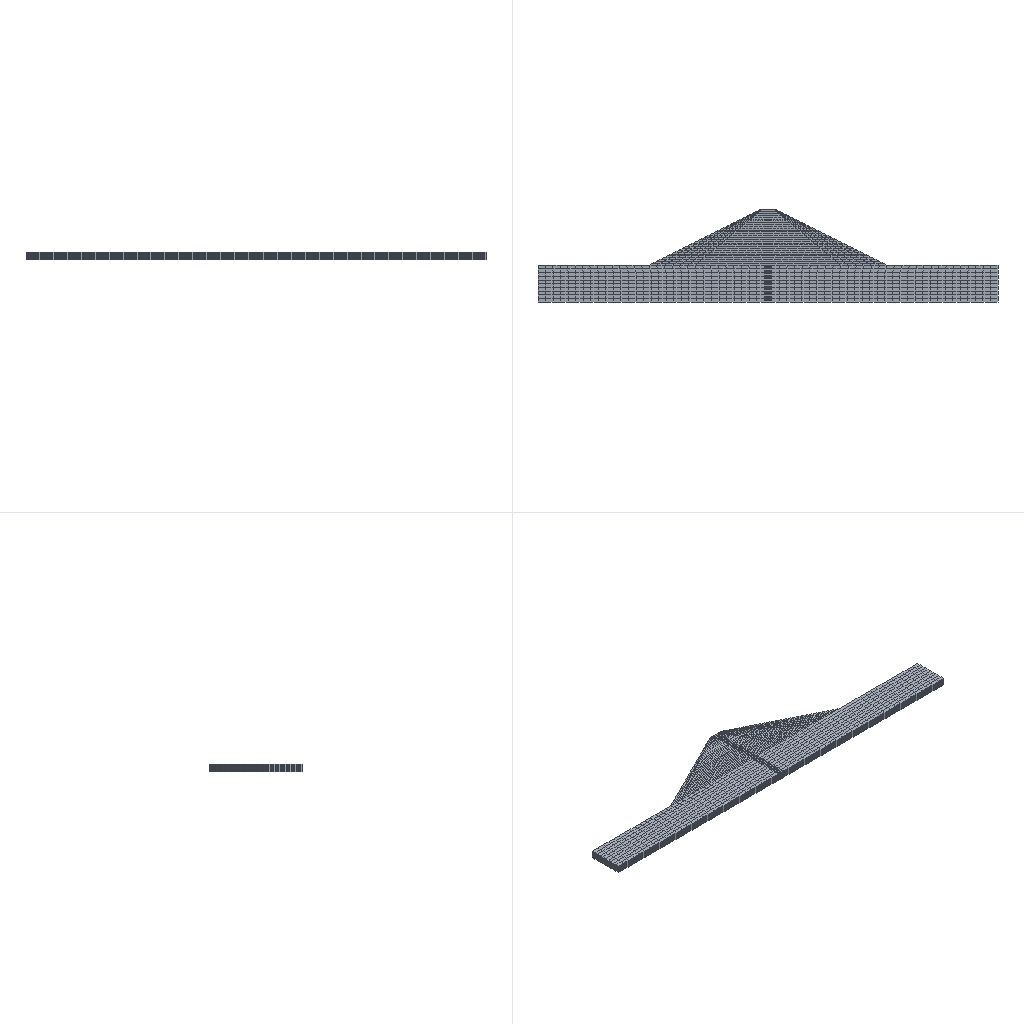Simulation study | abaqus
Set-up summary:
category,name,step,type,value,unit,region
solver,abaqus
solver,version,,,Abaqus/Standard 2020
units,not stated in the deck,,not stated
analysis,deck,,soils,soils
load_step,shenliu,shenliu,soils
load_step,requested,,,1
mesh,nodes,,,22968
mesh,elements,,,19240
element_type,C3D8P,,solid,19240
load,load commands in deck,,count,299
bc,support commands in deck,,count,313
material,BAJI,,in results
material,BATI,,in results
material,QIANG,,in results
check,setup vs results,,match,"per instance, exact: element labels, types and connectivity; labels of the nodes the elements use; coordinates of those nodes at SINGLE_PRECISION in 2 of 2 instance(s)"
Abaqus input file, long lists of numbers shortened:
*Heading
** Job name: Job-9 Model name: 3cm14mML300-OH-shenliu
** Generated by: Abaqus/CAE 2020
*Preprint, echo=NO, model=NO, history=NO, contact=NO
**
** PARTS
**
*Part, name=ba
*End Part
**
*Part, name=qiang
*End Part
**
**
** ASSEMBLY
**
*Assembly, name=Assembly
**
*Instance, name=ba-1, part=ba
*Node
      1,         67.5,         23.5,   1.2
      2,         67.5,         23.5,  0.9
** (22570 more lines like these left out)
*Element, type=C3D8P
 1,   208,  2707, 12325,  2651,     1,   169,  2647,   174
 2,  2707,   236,  2679, 12325,   169,     2,   170,  2647
** (19078 more lines like these left out)
*Nset, nset=Set-1
     1,     2,     3,     4,     5,     6,     7,     8,     9,    10,    11,    12,    13,    14,    15,    16
    17,    18,    19,    20,    21,    22,    23,    24,    25,    26,    27,    28,    29,    30,    31,    32
** (894 more lines like these left out)
*Elset, elset=Set-1
     1,     2,     3,     4,     5,     6,     7,     8,     9,    10,    11,    12,    13,    14,    15,    16
    17,    18,    19,    20,    21,    22,    23,    24,    25,    26,    27,    28,    29,    30,    31,    32
** (748 more lines like these left out)
*Nset, nset=Set-2
    18,    19,    21,    22,    24,    25,    26,    27,    41,    42,    44,    45,    56,    57,    59,    60
    75,    76,    77,    78,    79,    80,    81,    82,    83,    84,    85,    86,    87,    88,    89,    90
** (543 more lines like these left out)
*Elset, elset=Set-2
  4849,  4850,  4851,  4852,  4853,  4854,  4855,  4856,  4857,  4858,  4859,  4860,  4861,  4862,  4863,  4864
  4865,  4866,  4867,  4868,  4869,  4870,  4871,  4872,  4873,  4874,  4875,  4876,  4877,  4878,  4879,  4880
** (441 more lines like these left out)
** Section: bati
*Solid Section, elset=Set-1, material=bati
,
** Section: baji
*Solid Section, elset=Set-2, material=baji
,
*End Instance
**
*Instance, name=qiang-1, part=qiang
      62.235,           8.,           0.
*Node
      1, 0.03,         15.5,           0.
      2, 0.03,         15.5,  0.9
** (394 more lines like these left out)
*Element, type=C3D8P
 1,   8,  87, 307, 115,   1,  33, 281,  86
 2,  87,   5, 113, 307,  33,   2,  34, 281
** (158 more lines like these left out)
*Nset, nset=Set-1, generate
   1,  396,    1
*Elset, elset=Set-1, generate
   1,  160,    1
** Section: qiang
*Solid Section, elset=Set-1, material=qiang
,
*End Instance
**
*Nset, nset=Set-1, instance=ba-1
    18,    19,    21,    22,    24,    25,    26,    27,    41,    42,    44,    45,    56,    57,    59,    60
    75,    76,    77,    78,    79,    80,    81,    82,    83,    84,    85,    86,    87,    88,    89,    90
** (543 more lines like these left out)
*Elset, elset=Set-1, instance=ba-1
  4849,  4850,  4851,  4852,  4853,  4854,  4855,  4856,  4857,  4858,  4859,  4860,  4861,  4862,  4863,  4864
  4865,  4866,  4867,  4868,  4869,  4870,  4871,  4872,  4873,  4874,  4875,  4876,  4877,  4878,  4879,  4880
** (441 more lines like these left out)
*Nset, nset=Set-2, instance=ba-1
   115,   116,   117,   118,   121,   122,   125,   126,   135,   136,   137,   138,   145,   146,   149,   150
   156,   157,   158,   159,   162,   163,   164,   165,  1335,  1336,  1337,  1338,  1444,  1445,  1446,  1447
** (14 more lines like these left out)
*Elset, elset=Set-2, instance=ba-1
  5525,  5526,  5527,  5528,  5761,  5762,  5763,  5764,  5765,  5766,  5767,  5768,  6001,  6002,  6003,  6004
  6005,  6006,  6007,  6008,  6553,  6554,  6555,  6556,  6557,  6558,  6559,  6560,  6561,  6562,  6563,  6564
** (11 more lines like these left out)
*Nset, nset=Set-3, instance=ba-1
    81,    82,    83,    84,    85,    88,    91,    92,    93,    94,    97,    98,   127,   128,   129,   130
   133,   134,   136,   137,   140,   141,   142,   144,   145,   147,   148,   150,   162,   163,   164,   165
** (48 more lines like these left out)
*Elset, elset=Set-3, instance=ba-1
  4877,  4878,  4879,  4880,  4881,  4889,  4897,  4905,  4927,  4928,  4929,  4930,  4931,  4932,  4933,  4934
  4935,  4936,  4937,  4938,  4939,  4940,  4941,  4942,  4943,  4944,  5057,  5058,  5059,  5060,  5061,  5062
** (43 more lines like these left out)
*Nset, nset=Set-4, instance=ba-1
    17,    19,    20,    22,    23,    25,    27,    28,    29,    30,    31,    32,    35,    36,    37,    38
    39,    40,    41,    42,    51,    52,    53,    54,    58,    60,    63,    64,    65,    66,    67,    68
** (255 more lines like these left out)
*Nset, nset=Set-4, instance=qiang-1
   1,   4,   7,   8,   9,  12,  15,  16,  22,  23,  27,  28,  29,  30,  31,  32
  61,  62,  63,  64,  65,  66,  67,  68,  69,  70,  71,  72,  73,  74,  75,  76
** (7 more lines like these left out)
*Elset, elset=Set-4, instance=ba-1
   181,   185,   189,   193,   197,   201,   205,   209,   213,   217,   221,   225,   229,   233,   237,   241
   245,   249,   253,   257,   261,   265,   269,   273,   277,   281,   285,   289,   293,   297,   301,   305
** (237 more lines like these left out)
*Elset, elset=Set-4, instance=qiang-1
   1,   3,   5,   7,   9,  11,  13,  15,  17,  19,  21,  23,  25,  27,  29,  31
  33,  35,  37,  39,  41,  43,  45,  47,  49,  51,  53,  55,  57,  59,  93,  94
** (2 more lines like these left out)
*Nset, nset=Set-6, instance=ba-1
     1,     2,     3,     4,     6,     7,    13,    14,    15,    16,    18,    19,    20,    21,    22,    24
    25,    26,    27,    28,    31,    32,    34,    36,    37,    41,    42,    44,    45,    49,    53,    56
** (599 more lines like these left out)
*Nset, nset=Set-6, instance=qiang-1
   1,   4,   7,   8,  11,  12,  14,  15,  17,  18,  21,  22,  23,  24,  25,  26
  29,  30,  31,  32,  61,  62,  63,  64,  65,  66,  67,  68,  69,  70,  71,  72
** (4 more lines like these left out)
*Elset, elset=Set-6, instance=ba-1
     1,     2,     3,     4,     5,     6,    11,    12,    17,    18,    23,    24,    29,    30,    35,    36
    41,    42,    47,    48,    53,    54,    59,    60,    65,    66,    71,    72,    77,    78,    83,    84
** (491 more lines like these left out)
*Elset, elset=Set-6, instance=qiang-1
   1,   3,   5,   7,   9,  11,  13,  15,  17,  19,  21,  23,  25,  27,  29,  31
  33,  35,  37,  39,  41,  43,  45,  47,  49,  51,  53,  59,  60,  63,  91,  93
** (1 more lines like these left out)
*Nset, nset=Set-7, instance=ba-1, generate
     1,  22572,      1
*Nset, nset=Set-7, instance=qiang-1, generate
   1,  396,    1
*Elset, elset=Set-7, instance=ba-1, generate
     1,  19080,      1
*Elset, elset=Set-7, instance=qiang-1, generate
   1,  160,    1
*Nset, nset=Set-8, instance=ba-1
    18,    19,    21,    22,    24,    25,    26,    27,    41,    42,    44,    45,    56,    57,    59,    60
    75,    76,    77,    78,    79,    80,    81,    82,    83,    84,    85,    86,    87,    88,    89,    90
** (543 more lines like these left out)
*Elset, elset=Set-8, instance=ba-1
  4849,  4850,  4851,  4852,  4853,  4854,  4855,  4856,  4857,  4858,  4859,  4860,  4861,  4862,  4863,  4864
  4865,  4866,  4867,  4868,  4869,  4870,  4871,  4872,  4873,  4874,  4875,  4876,  4877,  4878,  4879,  4880
** (441 more lines like these left out)
*Nset, nset=Set-9, instance=ba-1
    18,    19,    21,    22,    24,    25,    26,    27,    41,    42,    44,    45,    56,    57,    59,    60
    75,    76,    77,    78,    79,    80,    81,    82,    83,    84,    85,    86,    87,    88,    89,    90
** (543 more lines like these left out)
*Elset, elset=Set-9, instance=ba-1
  4849,  4850,  4851,  4852,  4853,  4854,  4855,  4856,  4857,  4858,  4859,  4860,  4861,  4862,  4863,  4864
  4865,  4866,  4867,  4868,  4869,  4870,  4871,  4872,  4873,  4874,  4875,  4876,  4877,  4878,  4879,  4880
** (441 more lines like these left out)
*Nset, nset=Set-10, instance=ba-1
    18,    19,    21,    22,    24,    25,    26,    27,    41,    42,    44,    45,    56,    57,    59,    60
    75,    76,    77,    78,    79,    80,    81,    82,    83,    84,    85,    86,    87,    88,    89,    90
** (543 more lines like these left out)
*Elset, elset=Set-10, instance=ba-1
  4849,  4850,  4851,  4852,  4853,  4854,  4855,  4856,  4857,  4858,  4859,  4860,  4861,  4862,  4863,  4864
  4865,  4866,  4867,  4868,  4869,  4870,  4871,  4872,  4873,  4874,  4875,  4876,  4877,  4878,  4879,  4880
** (441 more lines like these left out)
*Nset, nset=Set-12, instance=ba-1
    13,    14,    20,    21,    22,    32,   119,   123,   243,   363,   364,   365,   366,   367,   368,   369
   370,   371,   372,   373,   374,   375,   376,   377,   378,   379,   380,   381,   382,   383,   384,   385
** (18 more lines like these left out)
*Elset, elset=Set-12, instance=ba-1
  1693,  1694,  1695,  1696,  1697,  1698,  1699,  1700,  1701,  1702,  1703,  1704,  1705,  1706,  1707,  1708
  1709,  1710,  1711,  1712,  1713,  1714,  1715,  1716,  1717,  1718,  1719,  1720,  1721,  1722,  1723,  1724
** (15 more lines like these left out)
*Nset, nset=Set-15, instance=ba-1
    18,    19,    21,    22,    24,    25,    26,    27,    41,    42,    44,    45,    56,    57,    59,    60
    75,    76,    77,    78,    79,    80,    81,    82,    83,    84,    85,    86,    87,    88,    89,    90
** (543 more lines like these left out)
*Elset, elset=Set-15, instance=ba-1
  4849,  4850,  4851,  4852,  4853,  4854,  4855,  4856,  4857,  4858,  4859,  4860,  4861,  4862,  4863,  4864
  4865,  4866,  4867,  4868,  4869,  4870,  4871,  4872,  4873,  4874,  4875,  4876,  4877,  4878,  4879,  4880
** (441 more lines like these left out)
*Nset, nset=Set-21, instance=ba-1
    18,    19,    21,    22,    24,    25,    26,    27,    41,    42,    44,    45,    56,    57,    59,    60
    75,    76,    77,    78,    79,    80,    81,    82,    83,    84,    85,    86,    87,    88,    89,    90
** (543 more lines like these left out)
*Elset, elset=Set-21, instance=ba-1
  4849,  4850,  4851,  4852,  4853,  4854,  4855,  4856,  4857,  4858,  4859,  4860,  4861,  4862,  4863,  4864
  4865,  4866,  4867,  4868,  4869,  4870,  4871,  4872,  4873,  4874,  4875,  4876,  4877,  4878,  4879,  4880
** (441 more lines like these left out)
*Nset, nset=Set-22, instance=ba-1
    18,    19,    21,    22,    24,    25,    26,    27,    41,    42,    44,    45,    56,    57,    59,    60
    75,    76,    77,    78,    79,    80,    81,    82,    83,    84,    85,    86,    87,    88,    89,    90
** (543 more lines like these left out)
*Elset, elset=Set-22, instance=ba-1
  4849,  4850,  4851,  4852,  4853,  4854,  4855,  4856,  4857,  4858,  4859,  4860,  4861,  4862,  4863,  4864
  4865,  4866,  4867,  4868,  4869,  4870,  4871,  4872,  4873,  4874,  4875,  4876,  4877,  4878,  4879,  4880
** (441 more lines like these left out)
*Nset, nset=Set-23, instance=ba-1, generate
     1,  22572,      1
*Nset, nset=Set-23, instance=qiang-1, generate
   1,  396,    1
*Elset, elset=Set-23, instance=ba-1, generate
     1,  19080,      1
*Elset, elset=Set-23, instance=qiang-1, generate
   1,  160,    1
*Elset, elset=_ba-xia_S2, internal, instance=ba-1
 4849, 4850, 4851, 4852, 4913, 4914
*Elset, elset=_ba-xia_S4, internal, instance=ba-1, generate
 4888,  4912,     8
*Surface, type=ELEMENT, name=ba-xia
_ba-xia_S2, S2
_ba-xia_S4, S4
*Elset, elset=_ba-you_S5, internal, instance=ba-1
  5261,  5262,  5263,  5264,  5277,  5278,  5279,  5280,  5325,  5326,  5327,  5328,  5341,  5342,  5343,  5344
  5383,  5384,  5391,  5392, 10983, 10984, 10985, 10986, 10999, 11000, 11001, 11002, 11015, 11016, 11017, 11018
** (13 more lines like these left out)
*Elset, elset=_ba-you_S4, internal, instance=ba-1, generate
 10510,  10722,      4
*Elset, elset=_ba-you_S2, internal, instance=ba-1, generate
 4549,  4554,     1
*Elset, elset=_ba-you_S6, internal, instance=ba-1, generate
 4435,  4527,     4
*Surface, type=ELEMENT, name=ba-you
_ba-you_S5, S5
_ba-you_S4, S4
_ba-you_S2, S2
_ba-you_S6, S6
*Elset, elset=_ba-zuo_S4, internal, instance=ba-1, generate
 3616,  4092,     4
*Elset, elset=_ba-zuo_S6, internal, instance=ba-1, generate
 4099,  4311,     4
*Elset, elset=_ba-zuo_S5, internal, instance=ba-1
 12101, 12102, 12109, 12110, 12117, 12118, 14105, 14106, 14107, 14108, 14121, 14122, 14123, 14124, 14137, 14138
 14139, 14140, 14153, 14154, 14155, 14156, 14169, 14170, 14171, 14172, 14185, 14186, 14187, 14188, 14201, 14202
** (6 more lines like these left out)
*Elset, elset=_ba-zuo_S1, internal, instance=ba-1
 5305, 5306, 5307, 5308, 5309, 5310, 5311, 5312, 5369, 5370, 5371, 5372, 5373, 5374, 5375, 5376
 5405, 5406, 5407, 5408
*Surface, type=ELEMENT, name=ba-zuo
_ba-zuo_S4, S4
_ba-zuo_S6, S6
_ba-zuo_S5, S5
_ba-zuo_S1, S1
*Elset, elset=_baxia_S1, internal, instance=ba-1
  3313,  3314,  3315,  3316,  3317,  3318,  3319,  3320,  3321,  3322,  3323,  3324,  3325,  3326,  3327,  3328
  3329,  3330,  3331,  3332,  3333,  3334,  3335,  3336,  3337,  3338,  3339,  3340,  3341,  3342,  3343,  3344
** (6 more lines like these left out)
*Elset, elset=_baxia_S2, internal, instance=ba-1, generate
 1,  6,  1
*Elset, elset=_baxia_S6, internal, instance=ba-1
  4555,  4570,  4585,  4600,  4615,  4630,  4645,  4660,  4675,  4690,  4705,  4720, 18271, 18286, 18301, 18316
 18331, 18346, 18361, 18376, 18391, 18406, 18421, 18436, 18451, 18466, 18481, 18496, 18511, 18526, 18541, 18556
** (3 more lines like these left out)
*Elset, elset=_baxia_S5, internal, instance=ba-1
  8691,  8692,  8693,  8694,  8751,  8752,  8753,  8754,  8811,  8812,  8813,  8814,  8871,  8872,  8873,  8874
  8931,  8932,  8933,  8934,  8991,  8992,  8993,  8994,  9051,  9052,  9053,  9054,  9111,  9112,  9113,  9114
** (5 more lines like these left out)
*Surface, type=ELEMENT, name=baxia
_baxia_S1, S1
_baxia_S2, S2
_baxia_S6, S6
_baxia_S5, S5
*Elset, elset=_fdown_S1, internal, instance=ba-1
  3313,  3314,  3315,  3316,  3317,  3318,  3319,  3320,  3321,  3322,  3323,  3324,  3325,  3326,  3327,  3328
  3329,  3330,  3331,  3332,  3333,  3334,  3335,  3336,  3337,  3338,  3339,  3340,  3341,  3342,  3343,  3344
** (6 more lines like these left out)
*Elset, elset=_fdown_S2, internal, instance=ba-1, generate
 1,  6,  1
*Elset, elset=_fdown_S6, internal, instance=ba-1
  4555,  4570,  4585,  4600,  4615,  4630,  4645,  4660,  4675,  4690,  4705,  4720, 18271, 18286, 18301, 18316
 18331, 18346, 18361, 18376, 18391, 18406, 18421, 18436, 18451, 18466, 18481, 18496, 18511, 18526, 18541, 18556
** (3 more lines like these left out)
*Elset, elset=_fdown_S5, internal, instance=ba-1
  8691,  8692,  8693,  8694,  8751,  8752,  8753,  8754,  8811,  8812,  8813,  8814,  8871,  8872,  8873,  8874
  8931,  8932,  8933,  8934,  8991,  8992,  8993,  8994,  9051,  9052,  9053,  9054,  9111,  9112,  9113,  9114
** (5 more lines like these left out)
*Surface, type=ELEMENT, name=fdown
_fdown_S1, S1
_fdown_S2, S2
_fdown_S6, S6
_fdown_S5, S5
*Elset, elset=_m_Surf-14_S4, internal, instance=ba-1, generate
 3616,  4092,     4
*Elset, elset=_m_Surf-14_S6, internal, instance=ba-1, generate
 4099,  4311,     4
*Elset, elset=_m_Surf-14_S5, internal, instance=ba-1
 12101, 12102, 12109, 12110, 12117, 12118, 14105, 14106, 14107, 14108, 14121, 14122, 14123, 14124, 14137, 14138
 14139, 14140, 14153, 14154, 14155, 14156, 14169, 14170, 14171, 14172, 14185, 14186, 14187, 14188, 14201, 14202
** (6 more lines like these left out)
*Elset, elset=_m_Surf-14_S1, internal, instance=ba-1
 5305, 5306, 5307, 5308, 5309, 5310, 5311, 5312, 5369, 5370, 5371, 5372, 5373, 5374, 5375, 5376
 5405, 5406, 5407, 5408
*Surface, type=ELEMENT, name=m_Surf-14
_m_Surf-14_S4, S4
_m_Surf-14_S6, S6
_m_Surf-14_S5, S5
_m_Surf-14_S1, S1
*Elset, elset=_m_Surf-16_S5, internal, instance=ba-1
  5261,  5262,  5263,  5264,  5277,  5278,  5279,  5280,  5325,  5326,  5327,  5328,  5341,  5342,  5343,  5344
  5383,  5384,  5391,  5392, 10983, 10984, 10985, 10986, 10999, 11000, 11001, 11002, 11015, 11016, 11017, 11018
** (13 more lines like these left out)
*Elset, elset=_m_Surf-16_S4, internal, instance=ba-1, generate
 10510,  10722,      4
*Elset, elset=_m_Surf-16_S2, internal, instance=ba-1, generate
 4549,  4554,     1
*Elset, elset=_m_Surf-16_S6, internal, instance=ba-1, generate
 4435,  4527,     4
*Surface, type=ELEMENT, name=m_Surf-16
_m_Surf-16_S5, S5
_m_Surf-16_S4, S4
_m_Surf-16_S2, S2
_m_Surf-16_S6, S6
*Elset, elset=_m_Surf-18_S2, internal, instance=ba-1
 4849, 4850, 4851, 4852, 4913, 4914
*Elset, elset=_m_Surf-18_S4, internal, instance=ba-1, generate
 4888,  4912,     8
*Surface, type=ELEMENT, name=m_Surf-18
_m_Surf-18_S2, S2
_m_Surf-18_S4, S4
*Elset, elset=_qiang-xia_S6, internal, instance=qiang-1
 91, 93
*Elset, elset=_qiang-xia_S4, internal, instance=qiang-1
  96, 158, 160
*Surface, type=ELEMENT, name=qiang-xia
_qiang-xia_S6, S6
_qiang-xia_S4, S4
*Elset, elset=_qiang-you_S2, internal, instance=qiang-1
   1,   2,   3,   4,   5,   6,   7,   8,   9,  10,  11,  12,  13,  14,  15,  16
  17,  18,  19,  20,  21,  22,  23,  24,  25,  26,  27,  28,  29,  30,  31,  32
** (8 more lines like these left out)
*Elset, elset=_qiang-you_S1, internal, instance=qiang-1
  91,  92,  93,  94,  95,  96, 157, 158, 159, 160
*Surface, type=ELEMENT, name=qiang-you
_qiang-you_S2, S2
_qiang-you_S1, S1
*Elset, elset=_qiang-zuo_S1, internal, instance=qiang-1
   1,   2,   3,   4,   5,   6,   7,   8,   9,  10,  11,  12,  13,  14,  15,  16
  17,  18,  19,  20,  21,  22,  23,  24,  25,  26,  27,  28,  29,  30,  31,  32
** (8 more lines like these left out)
*Elset, elset=_qiang-zuo_S2, internal, instance=qiang-1
  91,  92,  93,  94,  95,  96, 157, 158, 159, 160
*Surface, type=ELEMENT, name=qiang-zuo
_qiang-zuo_S1, S1
_qiang-zuo_S2, S2
*Elset, elset=_qiangdi_S5, internal, instance=qiang-1
  59,  60,  63, 155, 156
*Surface, type=ELEMENT, name=qiangdi
_qiangdi_S5, S5
*Elset, elset=_s_Surf-14_S1, internal, instance=qiang-1
   1,   2,   3,   4,   5,   6,   7,   8,   9,  10,  11,  12,  13,  14,  15,  16
  17,  18,  19,  20,  21,  22,  23,  24,  25,  26,  27,  28,  29,  30,  31,  32
** (8 more lines like these left out)
*Elset, elset=_s_Surf-14_S2, internal, instance=qiang-1
  91,  92,  93,  94,  95,  96, 157, 158, 159, 160
*Surface, type=ELEMENT, name=s_Surf-14
_s_Surf-14_S1, S1
_s_Surf-14_S2, S2
*Elset, elset=_s_Surf-16_S2, internal, instance=qiang-1
   1,   2,   3,   4,   5,   6,   7,   8,   9,  10,  11,  12,  13,  14,  15,  16
  17,  18,  19,  20,  21,  22,  23,  24,  25,  26,  27,  28,  29,  30,  31,  32
** (8 more lines like these left out)
*Elset, elset=_s_Surf-16_S1, internal, instance=qiang-1
  91,  92,  93,  94,  95,  96, 157, 158, 159, 160
*Surface, type=ELEMENT, name=s_Surf-16
_s_Surf-16_S2, S2
_s_Surf-16_S1, S1
*Elset, elset=_s_Surf-18_S6, internal, instance=qiang-1
 91, 93
*Elset, elset=_s_Surf-18_S4, internal, instance=qiang-1
  96, 158, 160
*Surface, type=ELEMENT, name=s_Surf-18
_s_Surf-18_S6, S6
_s_Surf-18_S4, S4
*Nset, nset=Set-12_PP_, internal, instance=ba-1
    13,    14,    20,    21,    22,    32,   119,   123,   243,   363,   364,   365,   366,   367,   368,   369
   370,   371,   372,   373,   374,   375,   376,   377,   378,   379,   380,   381,   382,   383,   384,   385
** (18 more lines like these left out)
*End Assembly
**
** MATERIALS
**
*Material, name=baji
*Density
2200.,
*Elastic
 2e+08, 0.29
*Permeability, specific=10000.
 1e-07, 1.5
*Material, name=bati
*Density
1930.,
*Elastic
 1e+08, 0.29
*Permeability, specific=10000.
 5e-07, 1.5
*Permeability, Type=SATURATION
     1e-05, 0.02154
    0.0001, 0.04642
     0.001,       0.1
 0.07244,  0.4169
  0.9703,      0.99
        1.,        1.
*Sorption
-200000., 0.02154
-150000., 0.04642
-100000.,       0.1
 -50000.,  0.4169
 -20000.,      0.99
      0.,        1.
*Material, name=qiang
*Density
300.,
*Elastic
 1.00176e+08, 0.272
*Permeability, specific=10000.
 1e-10, 1.5
**
** INTERACTION PROPERTIES
**
*Surface Interaction, name=IntProp-1
1.,
*Friction, slip tolerance=0.005
 0.1,
*Surface Behavior, penalty
*Surface Interaction, name=goodman
1.,
*Friction, user, depvar=1, properties=7
300.,   300.,   0.34,   0.95,   11.3, 10000.,100000.
*Surface Behavior, pressure-overclosure=HARD
**
** BOUNDARY CONDITIONS
**
** Name: x Type: Displacement/Rotation
*Boundary
Set-2, 1, 1
** Name: y Type: Displacement/Rotation
*Boundary
Set-3, 1, 1
Set-3, 2, 2
Set-3, 3, 3
** Name: z Type: Displacement/Rotation
*Boundary
Set-4, 3, 3
** PREDEFINED FIELDS
**
** Name: Predefined Field-1   Type: Saturation
*Initial Conditions, type=SATURATION
Set-7, 1.
** Name: Predefined Field-2   Type: Void ratio
*Initial Conditions, TYPE=RATIO
Set-7, 1.
**
** INTERACTIONS
**
** Interaction: xia
*Contact Pair, interaction=IntProp-1, type=SURFACE TO SURFACE
qiang-xia, ba-xia
** Interaction: you
*Contact Pair, interaction=IntProp-1, type=SURFACE TO SURFACE
qiang-you, ba-you
** Interaction: zuo
*Contact Pair, interaction=IntProp-1, type=SURFACE TO SURFACE
qiang-zuo, ba-zuo
** ----------------------------------------------------------------
**
** STEP: shenliu
**
*Step, name=shenliu, nlgeom=NO, inc=1000
*Soils, utol=1.0, creep=none
0.1, 1., 1e-05, 1.,
*sflow
fdown,qd,0.1
**
** BOUNDARY CONDITIONS
**
** Name: shenliu Type: Pore pressure Using Analytical Field: shenliu135
*Boundary
ba-1.13, 8, 8, 0.
ba-1.14, 8, 8, 0.
ba-1.20, 8, 8, 0.
ba-1.21, 8, 8, 135000.
ba-1.22, 8, 8, 135000.
ba-1.32, 8, 8, 0.
ba-1.119, 8, 8, 135000.
ba-1.123, 8, 8, 135000.
ba-1.243, 8, 8, 0.
ba-1.363, 8, 8, 0.
ba-1.364, 8, 8, 0.
ba-1.365, 8, 8, 0.
ba-1.366, 8, 8, 5000.
ba-1.367, 8, 8, 10000.
ba-1.368, 8, 8, 15000.
ba-1.369, 8, 8, 20000.
ba-1.370, 8, 8, 25000.
ba-1.371, 8, 8, 30000.
ba-1.372, 8, 8, 35000.
ba-1.373, 8, 8, 40000.
ba-1.374, 8, 8, 45000.
ba-1.375, 8, 8, 50000.
ba-1.376, 8, 8, 55000.
ba-1.377, 8, 8, 60000.
ba-1.378, 8, 8, 65000.
ba-1.379, 8, 8, 70000.
ba-1.380, 8, 8, 75000.
ba-1.381, 8, 8, 80000.
ba-1.382, 8, 8, 85000.
ba-1.383, 8, 8, 90000.
ba-1.384, 8, 8, 95000.
ba-1.385, 8, 8, 100000.
ba-1.386, 8, 8, 105000.
ba-1.387, 8, 8, 110000.
ba-1.388, 8, 8, 115000.
ba-1.389, 8, 8, 120000.
ba-1.390, 8, 8, 125000.
ba-1.391, 8, 8, 130000.
ba-1.392, 8, 8, 135000.
ba-1.393, 8, 8, 135000.
** (268 more lines like these left out)
**
** LOADS
**
** Name: Load-2   Type: Gravity
*Dload
, GRAV, 9.8, 0., -1., 0.
**
** OUTPUT REQUESTS
**
*Restart, write, frequency=0
**
** FIELD OUTPUT: F-Output-2
**
*Output, field
*Node Output
POR, U
*Element Output, directions=YES
E, MISES, PEMAG, S, SAT, VOIDR
**
** HISTORY OUTPUT: H-Output-3
**
*Output, history
*Energy Output
ALLAE,
*End Step
Results summary:
result,step,,partial,increments=0 time=0.0/1.0
result,analysis,,,soils
result,last_loadstep,,,1
result,primary field,,,"U, POR"